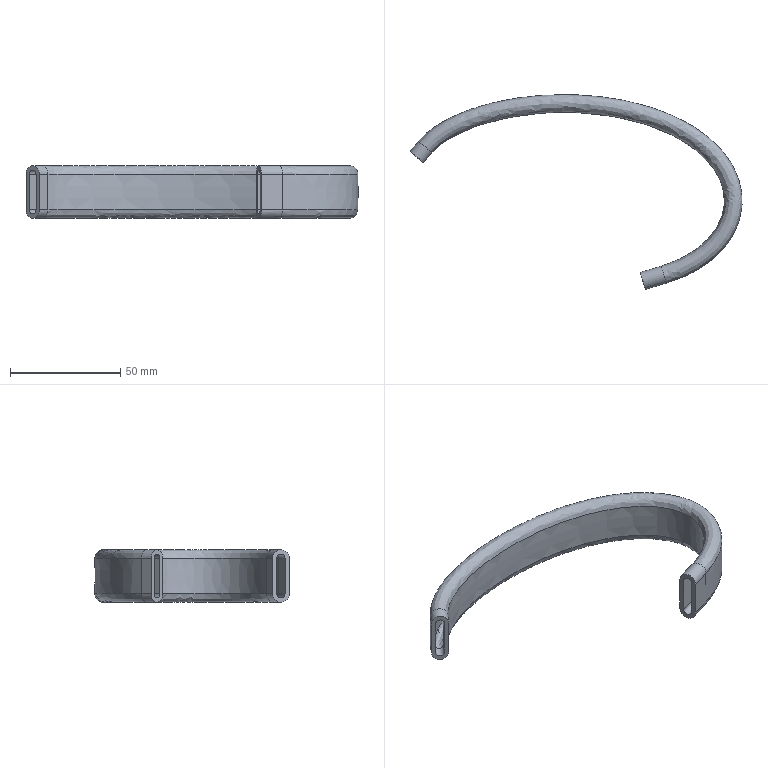Part | NX | features BREP 1 | 1 solid | 26 faces | box 150.882 x 88.437 x 24 mm | volume 23411 mm3 | plane 10 | spline 8 | cylinder 8 | commonest cylinder face diameters 4 x4 8 x4